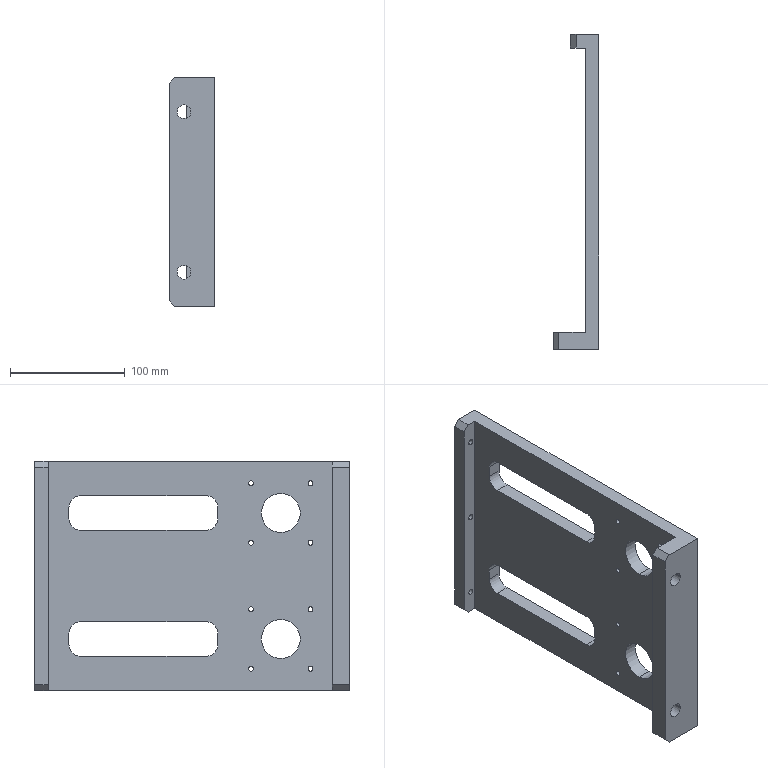Part | STEP file | Bracket | 1 solid | 60 faces | box 40 x 275 x 200 mm | volume 655765 mm3 | cylinder 38 | plane 22 | commonest cylinder face diameters 4.2 x16 20 x8 5 x6 12 x4 34 x4